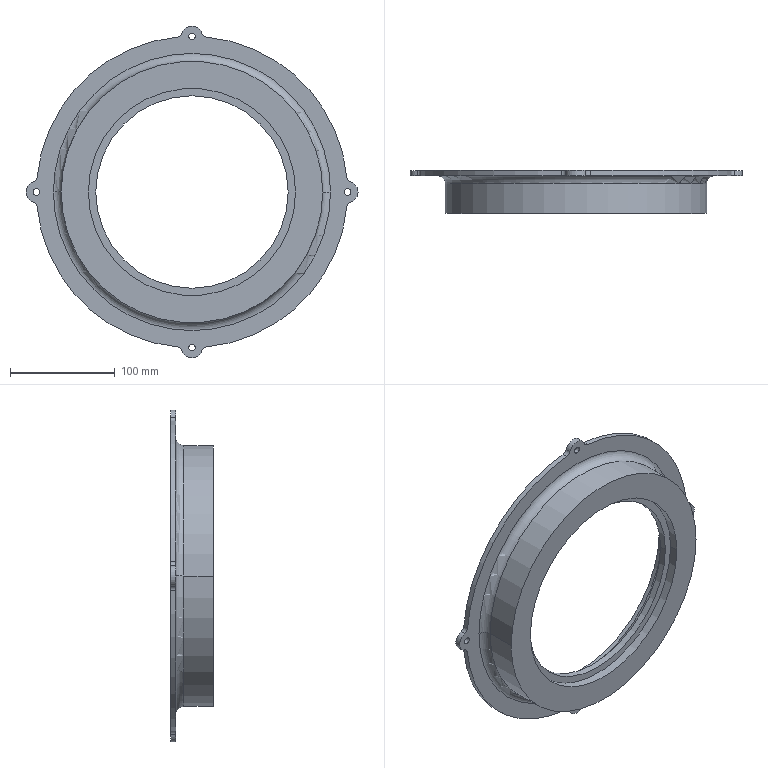Part | SolidWorks | features Cut 2, Fillet 2, ICE 2, Revolution 1 | 1 solid | 60 faces | box 317.492 x 41 x 317.492 mm | volume 402589 mm3 | cylinder 49 | plane 9 | torus 2 | commonest cylinder face diameters 2 x8 6.3 x8 10 x8 20 x5 242 x4 297.492 x4